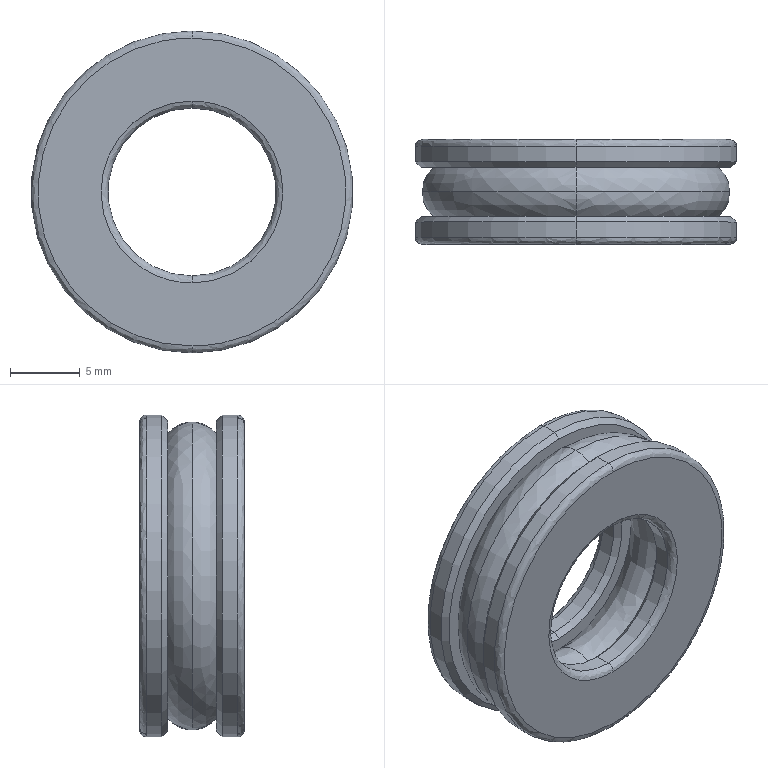Part | SolidWorks | features BaseBody 1 | 1 solid | 36 faces | box 23 x 7.5 x 23 mm | volume 1948 mm3 | spline 14 | cylinder 8 | cone 8 | plane 6 | commonest cylinder face diameters 12 x4 23 x4
STEP:
#1=CARTESIAN_POINT('',(0.,0.5,-6.));
#2=VERTEX_POINT('',#1);
#3=CARTESIAN_POINT('',(0.,0.5,6.));
#4=VERTEX_POINT('',#3);
#5=CARTESIAN_POINT('',(0.,0.5,0.));
#6=DIRECTION('',(0.,1.,0.));
#7=DIRECTION('',(0.,0.,-1.));
#8=AXIS2_PLACEMENT_3D('',#5,#6,#7);
#9=CIRCLE('',#8,6.);
#10=EDGE_CURVE('',#2,#4,#9,.T.);
#11=ORIENTED_EDGE('',*,*,#10,.T.);
#12=CARTESIAN_POINT('',(0.,0.,6.5));
#13=VERTEX_POINT('',#12);
#14=CARTESIAN_POINT('',(0.,0.5,6.5));
#15=DIRECTION('',(-1.,0.,0.));
#16=DIRECTION('',(0.,0.,1.));
#17=AXIS2_PLACEMENT_3D('',#14,#15,#16);
#18=CIRCLE('',#17,0.5);
#19=EDGE_CURVE('',#4,#13,#18,.T.);
#20=ORIENTED_EDGE('',*,*,#19,.T.);
#21=CARTESIAN_POINT('',(0.,0.,-6.5));
#22=VERTEX_POINT('',#21);
#23=CARTESIAN_POINT('',(0.,0.,6.5));
#24=CARTESIAN_POINT('',(-13.,0.,6.5));
#25=CARTESIAN_POINT('',(-13.,0.,-6.5));
#26=CARTESIAN_POINT('',(0.,0.,-6.5));
#27=(BOUNDED_CURVE()B_SPLINE_CURVE(3,(#23,#24,#25,#26),.UNSPECIFIED.,.F.,.F.)B_SPLINE_CURVE_WITH_KNOTS((4,4),(0.,1.),.UNSPECIFIED.)CURVE()GEOMETRIC_REPRESENTATION_ITEM()RATIONAL_B_SPLINE_CURVE((1.,0.3333,0.3333,1.))REPRESENTATION_ITEM(''));
#28=EDGE_CURVE('',#13,#22,#27,.T.);
#29=ORIENTED_EDGE('',*,*,#28,.T.);
#30=CARTESIAN_POINT('',(0.,0.5,-6.5));
#31=DIRECTION('',(1.,0.,0.));
#32=DIRECTION('',(0.,0.,-1.));
#33=AXIS2_PLACEMENT_3D('',#30,#31,#32);
#34=CIRCLE('',#33,0.5);
#35=EDGE_CURVE('',#2,#22,#34,.T.);
#36=ORIENTED_EDGE('',*,*,#35,.F.);
#37=EDGE_LOOP('',(#11,#20,#29,#36));
#38=FACE_OUTER_BOUND('',#37,.T.);
#39=CARTESIAN_POINT('',(0.,0.5,6.));
#40=CARTESIAN_POINT('',(-12.,0.5,6.));
#41=CARTESIAN_POINT('',(-12.,0.5,-6.));
#42=CARTESIAN_POINT('',(0.,0.5,-6.));
#43=CARTESIAN_POINT('',(0.,0.2071,6.));
#44=CARTESIAN_POINT('',(-12.,0.2071,6.));
#45=CARTESIAN_POINT('',(-12.,0.2071,-6.));
#46=CARTESIAN_POINT('',(0.,0.2071,-6.));
#47=CARTESIAN_POINT('',(0.,0.,6.207));
#48=CARTESIAN_POINT('',(-12.414,0.,6.207));
#49=CARTESIAN_POINT('',(-12.414,0.,-6.207));
#50=CARTESIAN_POINT('',(0.,0.,-6.207));
#51=CARTESIAN_POINT('',(0.,0.,6.5));
#52=CARTESIAN_POINT('',(-13.,0.,6.5));
#53=CARTESIAN_POINT('',(-13.,0.,-6.5));
#54=CARTESIAN_POINT('',(0.,0.,-6.5));
#55=(BOUNDED_SURFACE()B_SPLINE_SURFACE(3,3,((#39,#40,#41,#42),(#43,#44,#45,#46),(#47,#48,#49,#50),(#51,#52,#53,#54)),.UNSPECIFIED.,.F.,.F.,.F.)B_SPLINE_SURFACE_WITH_KNOTS((4,4),(4,4),(0.,1.),(0.,1.),.UNSPECIFIED.)GEOMETRIC_REPRESENTATION_ITEM()RATIONAL_B_SPLINE_SURFACE(((1.,0.3333,0.3333,1.),(0.8047,0.2682,0.2682,0.8047),(0.8047,0.2682,0.2682,0.8047),(1.,0.3333,0.3333,1.)))REPRESENTATION_ITEM('')SURFACE());
#56=ADVANCED_FACE('',(#38),#55,.T.);
#57=CARTESIAN_POINT('',(0.,0.,-11.));
#58=VERTEX_POINT('',#57);
#59=CARTESIAN_POINT('',(0.,0.,11.));
#60=VERTEX_POINT('',#59);
#61=CARTESIAN_POINT('',(0.,0.,-11.));
#62=CARTESIAN_POINT('',(-22.,0.,-11.));
#63=CARTESIAN_POINT('',(-22.,0.,11.));
#64=CARTESIAN_POINT('',(0.,0.,11.));
#65=(BOUNDED_CURVE()B_SPLINE_CURVE(3,(#61,#62,#63,#64),.UNSPECIFIED.,.F.,.F.)B_SPLINE_CURVE_WITH_KNOTS((4,4),(0.,1.),.UNSPECIFIED.)CURVE()GEOMETRIC_REPRESENTATION_ITEM()RATIONAL_B_SPLINE_CURVE((1.,0.3333,0.3333,1.))REPRESENTATION_ITEM(''));
#66=EDGE_CURVE('',#58,#60,#65,.T.);
#67=ORIENTED_EDGE('',*,*,#66,.T.);
#68=CARTESIAN_POINT('',(0.,0.5,11.5));
#69=VERTEX_POINT('',#68);
#70=CARTESIAN_POINT('',(0.,0.5,11.));
#71=DIRECTION('',(-1.,0.,0.));
#72=DIRECTION('',(0.,0.,1.));
#73=AXIS2_PLACEMENT_3D('',#70,#71,#72);
#74=CIRCLE('',#73,0.5);
#75=EDGE_CURVE('',#60,#69,#74,.T.);
#76=ORIENTED_EDGE('',*,*,#75,.T.);
#77=CARTESIAN_POINT('',(0.,0.5,-11.5));
#78=VERTEX_POINT('',#77);
#79=CARTESIAN_POINT('',(0.,0.5,0.));
#80=DIRECTION('',(0.,-1.,0.));
#81=DIRECTION('',(0.,0.,-1.));
#82=AXIS2_PLACEMENT_3D('',#79,#80,#81);
#83=CIRCLE('',#82,11.5);
#84=EDGE_CURVE('',#69,#78,#83,.T.);
#85=ORIENTED_EDGE('',*,*,#84,.T.);
#86=CARTESIAN_POINT('',(0.,0.5,-11.));
#87=DIRECTION('',(1.,0.,0.));
#88=DIRECTION('',(0.,0.,-1.));
#89=AXIS2_PLACEMENT_3D('',#86,#87,#88);
#90=CIRCLE('',#89,0.5);
#91=EDGE_CURVE('',#58,#78,#90,.T.);
#92=ORIENTED_EDGE('',*,*,#91,.F.);
#93=EDGE_LOOP('',(#67,#76,#85,#92));
#94=FACE_OUTER_BOUND('',#93,.T.);
#95=CARTESIAN_POINT('',(0.,0.,11.));
#96=CARTESIAN_POINT('',(-22.,0.,11.));
#97=CARTESIAN_POINT('',(-22.,0.,-11.));
#98=CARTESIAN_POINT('',(0.,0.,-11.));
#99=CARTESIAN_POINT('',(0.,0.,11.293));
#100=CARTESIAN_POINT('',(-22.586,0.,11.293));
#101=CARTESIAN_POINT('',(-22.586,0.,-11.293));
#102=CARTESIAN_POINT('',(0.,0.,-11.293));
#103=CARTESIAN_POINT('',(0.,0.2071,11.5));
#104=CARTESIAN_POINT('',(-23.,0.2071,11.5));
#105=CARTESIAN_POINT('',(-23.,0.2071,-11.5));
#106=CARTESIAN_POINT('',(0.,0.2071,-11.5));
#107=CARTESIAN_POINT('',(0.,0.5,11.5));
#108=CARTESIAN_POINT('',(-23.,0.5,11.5));
#109=CARTESIAN_POINT('',(-23.,0.5,-11.5));
#110=CARTESIAN_POINT('',(0.,0.5,-11.5));
#111=(BOUNDED_SURFACE()B_SPLINE_SURFACE(3,3,((#95,#96,#97,#98),(#99,#100,#101,#102),(#103,#104,#105,#106),(#107,#108,#109,#110)),.UNSPECIFIED.,.F.,.F.,.F.)B_SPLINE_SURFACE_WITH_KNOTS((4,4),(4,4),(0.,1.),(0.,1.),.UNSPECIFIED.)GEOMETRIC_REPRESENTATION_ITEM()RATIONAL_B_SPLINE_SURFACE(((1.,0.3333,0.3333,1.),(0.8047,0.2682,0.2682,0.8047),(0.8047,0.2682,0.2682,0.8047),(1.,0.3333,0.3333,1.)))REPRESENTATION_ITEM('')SURFACE());
#112=ADVANCED_FACE('',(#94),#111,.T.);
#113=CARTESIAN_POINT('',(0.,5.5,7.336));
#114=VERTEX_POINT('',#113);
#115=CARTESIAN_POINT('',(0.,5.5,-7.336));
#116=VERTEX_POINT('',#115);
#117=CARTESIAN_POINT('',(0.,5.5,0.));
#118=DIRECTION('',(0.,1.,0.));
#119=DIRECTION('',(0.,0.,-1.));
#120=AXIS2_PLACEMENT_3D('',#117,#118,#119);
#121=CIRCLE('',#120,7.336);
#122=EDGE_CURVE('',#114,#116,#121,.T.);
#123=ORIENTED_EDGE('',*,*,#122,.T.);
#124=CARTESIAN_POINT('',(0.,2.,-7.336));
#125=VERTEX_POINT('',#124);
#126=CARTESIAN_POINT('',(0.,3.75,-8.75));
#127=DIRECTION('',(1.,0.,0.));
#128=DIRECTION('',(0.,0.,-1.));
#129=AXIS2_PLACEMENT_3D('',#126,#127,#128);
#130=CIRCLE('',#129,2.25);
#131=EDGE_CURVE('',#116,#125,#130,.T.);
#132=ORIENTED_EDGE('',*,*,#131,.T.);
#133=CARTESIAN_POINT('',(0.,2.,7.336));
#134=VERTEX_POINT('',#133);
#135=CARTESIAN_POINT('',(0.,2.,0.));
#136=DIRECTION('',(0.,1.,0.));
#137=DIRECTION('',(0.,0.,-1.));
#138=AXIS2_PLACEMENT_3D('',#135,#136,#137);
#139=CIRCLE('',#138,7.336);
#140=EDGE_CURVE('',#134,#125,#139,.T.);
#141=ORIENTED_EDGE('',*,*,#140,.F.);
#142=CARTESIAN_POINT('',(0.,3.75,8.75));
#143=DIRECTION('',(-1.,0.,0.));
#144=DIRECTION('',(0.,0.,1.));
#145=AXIS2_PLACEMENT_3D('',#142,#143,#144);
#146=CIRCLE('',#145,2.25);
#147=EDGE_CURVE('',#114,#134,#146,.T.);
#148=ORIENTED_EDGE('',*,*,#147,.F.);
#149=EDGE_LOOP('',(#123,#132,#141,#148));
#150=FACE_OUTER_BOUND('',#149,.T.);
#151=CARTESIAN_POINT('',(0.,5.5,-7.336));
#152=CARTESIAN_POINT('',(14.672,5.5,-7.336));
#153=CARTESIAN_POINT('',(14.672,5.5,7.336));
#154=CARTESIAN_POINT('',(0.,5.5,7.336));
#155=CARTESIAN_POINT('',(0.,4.525,-6.13));
#156=CARTESIAN_POINT('',(12.259,4.525,-6.13));
#157=CARTESIAN_POINT('',(12.259,4.525,6.13));
#158=CARTESIAN_POINT('',(0.,4.525,6.13));
#159=CARTESIAN_POINT('',(0.,2.975,-6.13));
#160=CARTESIAN_POINT('',(12.259,2.975,-6.13));
#161=CARTESIAN_POINT('',(12.259,2.975,6.13));
#162=CARTESIAN_POINT('',(0.,2.975,6.13));
#163=CARTESIAN_POINT('',(0.,2.,-7.336));
#164=CARTESIAN_POINT('',(14.672,2.,-7.336));
#165=CARTESIAN_POINT('',(14.672,2.,7.336));
#166=CARTESIAN_POINT('',(0.,2.,7.336));
#167=(BOUNDED_SURFACE()B_SPLINE_SURFACE(3,3,((#151,#152,#153,#154),(#155,#156,#157,#158),(#159,#160,#161,#162),(#163,#164,#165,#166)),.UNSPECIFIED.,.F.,.F.,.F.)B_SPLINE_SURFACE_WITH_KNOTS((4,4),(4,4),(0.,1.),(0.,1.),.UNSPECIFIED.)GEOMETRIC_REPRESENTATION_ITEM()RATIONAL_B_SPLINE_SURFACE(((1.,0.3333,0.3333,1.),(0.7524,0.2508,0.2508,0.7524),(0.7524,0.2508,0.2508,0.7524),(1.,0.3333,0.3333,1.)))REPRESENTATION_ITEM('')SURFACE());
#168=ADVANCED_FACE('',(#150),#167,.T.);
#169=CARTESIAN_POINT('',(0.,3.75,11.));
#170=VERTEX_POINT('',#169);
#171=CARTESIAN_POINT('',(0.,3.75,-11.));
#172=VERTEX_POINT('',#171);
#173=CARTESIAN_POINT('',(0.,3.75,0.));
#174=DIRECTION('',(0.,-1.,0.));
#175=DIRECTION('',(0.,0.,-1.));
#176=AXIS2_PLACEMENT_3D('',#173,#174,#175);
#177=CIRCLE('',#176,11.);
#178=EDGE_CURVE('',#170,#172,#177,.T.);
#179=ORIENTED_EDGE('',*,*,#178,.F.);
#180=CARTESIAN_POINT('',(0.,5.5,10.164));
#181=VERTEX_POINT('',#180);
#182=CARTESIAN_POINT('',(0.,3.75,8.75));
#183=DIRECTION('',(-1.,0.,0.));
#184=DIRECTION('',(0.,0.,1.));
#185=AXIS2_PLACEMENT_3D('',#182,#183,#184);
#186=CIRCLE('',#185,2.25);
#187=EDGE_CURVE('',#170,#181,#186,.T.);
#188=ORIENTED_EDGE('',*,*,#187,.T.);
#189=CARTESIAN_POINT('',(0.,5.5,-10.164));
#190=VERTEX_POINT('',#189);
#191=CARTESIAN_POINT('',(0.,5.5,0.));
#192=DIRECTION('',(0.,-1.,0.));
#193=DIRECTION('',(0.,0.,-1.));
#194=AXIS2_PLACEMENT_3D('',#191,#192,#193);
#195=CIRCLE('',#194,10.164);
#196=EDGE_CURVE('',#181,#190,#195,.T.);
#197=ORIENTED_EDGE('',*,*,#196,.T.);
#198=CARTESIAN_POINT('',(0.,3.75,-8.75));
#199=DIRECTION('',(1.,0.,0.));
#200=DIRECTION('',(0.,0.,-1.));
#201=AXIS2_PLACEMENT_3D('',#198,#199,#200);
#202=CIRCLE('',#201,2.25);
#203=EDGE_CURVE('',#172,#190,#202,.T.);
#204=ORIENTED_EDGE('',*,*,#203,.F.);
#205=EDGE_LOOP('',(#179,#188,#197,#204));
#206=FACE_OUTER_BOUND('',#205,.T.);
#207=CARTESIAN_POINT('',(0.,3.75,11.));
#208=CARTESIAN_POINT('',(-22.,3.75,11.));
#209=CARTESIAN_POINT('',(-22.,3.75,-11.));
#210=CARTESIAN_POINT('',(0.,3.75,-11.));
#211=CARTESIAN_POINT('',(0.,4.441,11.));
#212=CARTESIAN_POINT('',(-22.,4.441,11.));
#213=CARTESIAN_POINT('',(-22.,4.441,-11.));
#214=CARTESIAN_POINT('',(0.,4.441,-11.));
#215=CARTESIAN_POINT('',(0.,5.065,10.702));
#216=CARTESIAN_POINT('',(-21.404,5.065,10.702));
#217=CARTESIAN_POINT('',(-21.404,5.065,-10.702));
#218=CARTESIAN_POINT('',(0.,5.065,-10.702));
#219=CARTESIAN_POINT('',(0.,5.5,10.164));
#220=CARTESIAN_POINT('',(-20.328,5.5,10.164));
#221=CARTESIAN_POINT('',(-20.328,5.5,-10.164));
#222=CARTESIAN_POINT('',(0.,5.5,-10.164));
#223=(BOUNDED_SURFACE()B_SPLINE_SURFACE(3,3,((#207,#208,#209,#210),(#211,#212,#213,#214),(#215,#216,#217,#218),(#219,#220,#221,#222)),.UNSPECIFIED.,.F.,.F.,.F.)B_SPLINE_SURFACE_WITH_KNOTS((4,4),(4,4),(0.,1.),(0.,1.),.UNSPECIFIED.)GEOMETRIC_REPRESENTATION_ITEM()RATIONAL_B_SPLINE_SURFACE(((1.,0.3333,0.3333,1.),(0.9349,0.3116,0.3116,0.9349),(0.9349,0.3116,0.3116,0.9349),(1.,0.3333,0.3333,1.)))REPRESENTATION_ITEM('')SURFACE());
#224=ADVANCED_FACE('',(#206),#223,.T.);
#225=CARTESIAN_POINT('',(0.,7.5,6.5));
#226=VERTEX_POINT('',#225);
#227=CARTESIAN_POINT('',(0.,7.5,-6.5));
#228=VERTEX_POINT('',#227);
#229=CARTESIAN_POINT('',(0.,7.5,6.5));
#230=CARTESIAN_POINT('',(13.,7.5,6.5));
#231=CARTESIAN_POINT('',(13.,7.5,-6.5));
#232=CARTESIAN_POINT('',(0.,7.5,-6.5));
#233=(BOUNDED_CURVE()B_SPLINE_CURVE(3,(#229,#230,#231,#232),.UNSPECIFIED.,.F.,.F.)B_SPLINE_CURVE_WITH_KNOTS((4,4),(0.,1.),.UNSPECIFIED.)CURVE()GEOMETRIC_REPRESENTATION_ITEM()RATIONAL_B_SPLINE_CURVE((1.,0.3333,0.3333,1.))REPRESENTATION_ITEM(''));
#234=EDGE_CURVE('',#226,#228,#233,.T.);
#235=ORIENTED_EDGE('',*,*,#234,.T.);
#236=CARTESIAN_POINT('',(0.,7.,-6.));
#237=VERTEX_POINT('',#236);
#238=CARTESIAN_POINT('',(0.,7.,-6.5));
#239=DIRECTION('',(1.,0.,0.));
#240=DIRECTION('',(0.,0.,-1.));
#241=AXIS2_PLACEMENT_3D('',#238,#239,#240);
#242=CIRCLE('',#241,0.5);
#243=EDGE_CURVE('',#228,#237,#242,.T.);
#244=ORIENTED_EDGE('',*,*,#243,.T.);
#245=CARTESIAN_POINT('',(0.,7.,6.));
#246=VERTEX_POINT('',#245);
#247=CARTESIAN_POINT('',(0.,7.,0.));
#248=DIRECTION('',(0.,-1.,0.));
#249=DIRECTION('',(0.,0.,-1.));
#250=AXIS2_PLACEMENT_3D('',#247,#248,#249);
#251=CIRCLE('',#250,6.);
#252=EDGE_CURVE('',#237,#246,#251,.T.);
#253=ORIENTED_EDGE('',*,*,#252,.T.);
#254=CARTESIAN_POINT('',(0.,7.,6.5));
#255=DIRECTION('',(-1.,0.,0.));
#256=DIRECTION('',(0.,0.,1.));
#257=AXIS2_PLACEMENT_3D('',#254,#255,#256);
#258=CIRCLE('',#257,0.5);
#259=EDGE_CURVE('',#226,#246,#258,.T.);
#260=ORIENTED_EDGE('',*,*,#259,.F.);
#261=EDGE_LOOP('',(#235,#244,#253,#260));
#262=FACE_OUTER_BOUND('',#261,.T.);
#263=CARTESIAN_POINT('',(0.,7.5,-6.5));
#264=CARTESIAN_POINT('',(13.,7.5,-6.5));
#265=CARTESIAN_POINT('',(13.,7.5,6.5));
#266=CARTESIAN_POINT('',(0.,7.5,6.5));
#267=CARTESIAN_POINT('',(0.,7.5,-6.207));
#268=CARTESIAN_POINT('',(12.414,7.5,-6.207));
#269=CARTESIAN_POINT('',(12.414,7.5,6.207));
#270=CARTESIAN_POINT('',(0.,7.5,6.207));
#271=CARTESIAN_POINT('',(0.,7.293,-6.));
#272=CARTESIAN_POINT('',(12.,7.293,-6.));
#273=CARTESIAN_POINT('',(12.,7.293,6.));
#274=CARTESIAN_POINT('',(0.,7.293,6.));
#275=CARTESIAN_POINT('',(0.,7.,-6.));
#276=CARTESIAN_POINT('',(12.,7.,-6.));
#277=CARTESIAN_POINT('',(12.,7.,6.));
#278=CARTESIAN_POINT('',(0.,7.,6.));
#279=(BOUNDED_SURFACE()B_SPLINE_SURFACE(3,3,((#263,#264,#265,#266),(#267,#268,#269,#270),(#271,#272,#273,#274),(#275,#276,#277,#278)),.UNSPECIFIED.,.F.,.F.,.F.)B_SPLINE_SURFACE_WITH_KNOTS((4,4),(4,4),(0.,1.),(0.,1.),.UNSPECIFIED.)GEOMETRIC_REPRESENTATION_ITEM()RATIONAL_B_SPLINE_SURFACE(((1.,0.3333,0.3333,1.),(0.8047,0.2682,0.2682,0.8047),(0.8047,0.2682,0.2682,0.8047),(1.,0.3333,0.3333,1.)))REPRESENTATION_ITEM('')SURFACE());
#280=ADVANCED_FACE('',(#262),#279,.T.);
#281=CARTESIAN_POINT('',(0.,7.,-11.5));
#282=VERTEX_POINT('',#281);
#283=CARTESIAN_POINT('',(0.,7.,11.5));
#284=VERTEX_POINT('',#283);
#285=CARTESIAN_POINT('',(0.,7.,0.));
#286=DIRECTION('',(0.,-1.,0.));
#287=DIRECTION('',(0.,0.,-1.));
#288=AXIS2_PLACEMENT_3D('',#285,#286,#287);
#289=CIRCLE('',#288,11.5);
#290=EDGE_CURVE('',#282,#284,#289,.T.);
#291=ORIENTED_EDGE('',*,*,#290,.F.);
#292=CARTESIAN_POINT('',(0.,7.5,-11.));
#293=VERTEX_POINT('',#292);
#294=CARTESIAN_POINT('',(0.,7.,-11.));
#295=DIRECTION('',(1.,0.,0.));
#296=DIRECTION('',(0.,0.,-1.));
#297=AXIS2_PLACEMENT_3D('',#294,#295,#296);
#298=CIRCLE('',#297,0.5);
#299=EDGE_CURVE('',#282,#293,#298,.T.);
#300=ORIENTED_EDGE('',*,*,#299,.T.);
#301=CARTESIAN_POINT('',(0.,7.5,11.));
#302=VERTEX_POINT('',#301);
#303=CARTESIAN_POINT('',(0.,7.5,-11.));
#304=CARTESIAN_POINT('',(22.,7.5,-11.));
#305=CARTESIAN_POINT('',(22.,7.5,11.));
#306=CARTESIAN_POINT('',(0.,7.5,11.));
#307=(BOUNDED_CURVE()B_SPLINE_CURVE(3,(#303,#304,#305,#306),.UNSPECIFIED.,.F.,.F.)B_SPLINE_CURVE_WITH_KNOTS((4,4),(0.,1.),.UNSPECIFIED.)CURVE()GEOMETRIC_REPRESENTATION_ITEM()RATIONAL_B_SPLINE_CURVE((1.,0.3333,0.3333,1.))REPRESENTATION_ITEM(''));
#308=EDGE_CURVE('',#293,#302,#307,.T.);
#309=ORIENTED_EDGE('',*,*,#308,.T.);
#310=CARTESIAN_POINT('',(0.,7.,11.));
#311=DIRECTION('',(-1.,0.,0.));
#312=DIRECTION('',(0.,0.,1.));
#313=AXIS2_PLACEMENT_3D('',#310,#311,#312);
#314=CIRCLE('',#313,0.5);
#315=EDGE_CURVE('',#284,#302,#314,.T.);
#316=ORIENTED_EDGE('',*,*,#315,.F.);
#317=EDGE_LOOP('',(#291,#300,#309,#316));
#318=FACE_OUTER_BOUND('',#317,.T.);
#319=CARTESIAN_POINT('',(0.,7.,-11.5));
#320=CARTESIAN_POINT('',(23.,7.,-11.5));
#321=CARTESIAN_POINT('',(23.,7.,11.5));
#322=CARTESIAN_POINT('',(0.,7.,11.5));
#323=CARTESIAN_POINT('',(0.,7.293,-11.5));
#324=CARTESIAN_POINT('',(23.,7.293,-11.5));
#325=CARTESIAN_POINT('',(23.,7.293,11.5));
#326=CARTESIAN_POINT('',(0.,7.293,11.5));
#327=CARTESIAN_POINT('',(0.,7.5,-11.293));
#328=CARTESIAN_POINT('',(22.586,7.5,-11.293));
#329=CARTESIAN_POINT('',(22.586,7.5,11.293));
#330=CARTESIAN_POINT('',(0.,7.5,11.293));
#331=CARTESIAN_POINT('',(0.,7.5,-11.));
#332=CARTESIAN_POINT('',(22.,7.5,-11.));
#333=CARTESIAN_POINT('',(22.,7.5,11.));
#334=CARTESIAN_POINT('',(0.,7.5,11.));
#335=(BOUNDED_SURFACE()B_SPLINE_SURFACE(3,3,((#319,#320,#321,#322),(#323,#324,#325,#326),(#327,#328,#329,#330),(#331,#332,#333,#334)),.UNSPECIFIED.,.F.,.F.,.F.)B_SPLINE_SURFACE_WITH_KNOTS((4,4),(4,4),(0.,1.),(0.,1.),.UNSPECIFIED.)GEOMETRIC_REPRESENTATION_ITEM()RATIONAL_B_SPLINE_SURFACE(((1.,0.3333,0.3333,1.),(0.8047,0.2682,0.2682,0.8047),(0.8047,0.2682,0.2682,0.8047),(1.,0.3333,0.3333,1.)))REPRESENTATION_ITEM('')SURFACE());
#336=ADVANCED_FACE('',(#318),#335,.T.);
#337=CARTESIAN_POINT('',(0.,2.,-10.164));
#338=VERTEX_POINT('',#337);
#339=CARTESIAN_POINT('',(0.,2.,10.164));
#340=VERTEX_POINT('',#339);
#341=CARTESIAN_POINT('',(0.,2.,0.));
#342=DIRECTION('',(0.,1.,0.));
#343=DIRECTION('',(0.,0.,-1.));
#344=AXIS2_PLACEMENT_3D('',#341,#342,#343);
#345=CIRCLE('',#344,10.164);
#346=EDGE_CURVE('',#338,#340,#345,.T.);
#347=ORIENTED_EDGE('',*,*,#346,.T.);
#348=CARTESIAN_POINT('',(0.,3.75,8.75));
#349=DIRECTION('',(-1.,0.,0.));
#350=DIRECTION('',(0.,0.,1.));
#351=AXIS2_PLACEMENT_3D('',#348,#349,#350);
#352=CIRCLE('',#351,2.25);
#353=EDGE_CURVE('',#340,#170,#352,.T.);
#354=ORIENTED_EDGE('',*,*,#353,.T.);
#355=ORIENTED_EDGE('',*,*,#178,.T.);
#356=CARTESIAN_POINT('',(0.,3.75,-8.75));
#357=DIRECTION('',(1.,0.,0.));
#358=DIRECTION('',(0.,0.,-1.));
#359=AXIS2_PLACEMENT_3D('',#356,#357,#358);
#360=CIRCLE('',#359,2.25);
#361=EDGE_CURVE('',#338,#172,#360,.T.);
#362=ORIENTED_EDGE('',*,*,#361,.F.);
#363=EDGE_LOOP('',(#347,#354,#355,#362));
#364=FACE_OUTER_BOUND('',#363,.T.);
#365=CARTESIAN_POINT('',(0.,2.,10.164));
#366=CARTESIAN_POINT('',(-20.328,2.,10.164));
#367=CARTESIAN_POINT('',(-20.328,2.,-10.164));
#368=CARTESIAN_POINT('',(0.,2.,-10.164));
#369=CARTESIAN_POINT('',(0.,2.435,10.702));
#370=CARTESIAN_POINT('',(-21.404,2.435,10.702));
#371=CARTESIAN_POINT('',(-21.404,2.435,-10.702));
#372=CARTESIAN_POINT('',(0.,2.435,-10.702));
#373=CARTESIAN_POINT('',(0.,3.059,11.));
#374=CARTESIAN_POINT('',(-22.,3.059,11.));
#375=CARTESIAN_POINT('',(-22.,3.059,-11.));
#376=CARTESIAN_POINT('',(0.,3.059,-11.));
#377=CARTESIAN_POINT('',(0.,3.75,11.));
#378=CARTESIAN_POINT('',(-22.,3.75,11.));
#379=CARTESIAN_POINT('',(-22.,3.75,-11.));
#380=CARTESIAN_POINT('',(0.,3.75,-11.));
#381=(BOUNDED_SURFACE()B_SPLINE_SURFACE(3,3,((#365,#366,#367,#368),(#369,#370,#371,#372),(#373,#374,#375,#376),(#377,#378,#379,#380)),.UNSPECIFIED.,.F.,.F.,.F.)B_SPLINE_SURFACE_WITH_KNOTS((4,4),(4,4),(0.,1.),(0.,1.),.UNSPECIFIED.)GEOMETRIC_REPRESENTATION_ITEM()RATIONAL_B_SPLINE_SURFACE(((1.,0.3333,0.3333,1.),(0.9349,0.3116,0.3116,0.9349),(0.9349,0.3116,0.3116,0.9349),(1.,0.3333,0.3333,1.)))REPRESENTATION_ITEM('')SURFACE());
#382=ADVANCED_FACE('',(#364),#381,.T.);
#383=CARTESIAN_POINT('',(0.,1.6,6.));
#384=VERTEX_POINT('',#383);
#385=CARTESIAN_POINT('',(0.,1.6,-6.));
#386=VERTEX_POINT('',#385);
#387=CARTESIAN_POINT('',(0.,1.6,0.));
#388=DIRECTION('',(0.,-1.,0.));
#389=DIRECTION('',(0.,0.,-1.));
#390=AXIS2_PLACEMENT_3D('',#387,#388,#389);
#391=CIRCLE('',#390,6.);
#392=EDGE_CURVE('',#384,#386,#391,.T.);
#393=ORIENTED_EDGE('',*,*,#392,.F.);
#394=CARTESIAN_POINT('',(0.,0.,6.));
#395=DIRECTION('',(0.,-1.,0.));
#396=VECTOR('',#395,1000.);
#397=LINE('',#394,#396);
#398=EDGE_CURVE('',#384,#4,#397,.T.);
#399=ORIENTED_EDGE('',*,*,#398,.T.);
#400=ORIENTED_EDGE('',*,*,#10,.F.);
#401=CARTESIAN_POINT('',(0.,0.,-6.));
#402=DIRECTION('',(0.,-1.,0.));
#403=VECTOR('',#402,1000.);
#404=LINE('',#401,#403);
#405=EDGE_CURVE('',#386,#2,#404,.T.);
#406=ORIENTED_EDGE('',*,*,#405,.F.);
#407=EDGE_LOOP('',(#393,#399,#400,#406));
#408=FACE_OUTER_BOUND('',#407,.T.);
#409=CARTESIAN_POINT('',(0.,0.,0.));
#410=DIRECTION('',(0.,-1.,0.));
#411=DIRECTION('',(0.,0.,-1.));
#412=AXIS2_PLACEMENT_3D('',#409,#410,#411);
#413=CYLINDRICAL_SURFACE('',#412,6.);
#414=ADVANCED_FACE('',(#408),#413,.F.);
#415=CARTESIAN_POINT('',(0.,1.6,-11.5));
#416=VERTEX_POINT('',#415);
#417=CARTESIAN_POINT('',(0.,1.6,11.5));
#418=VERTEX_POINT('',#417);
#419=CARTESIAN_POINT('',(0.,1.6,0.));
#420=DIRECTION('',(0.,-1.,0.));
#421=DIRECTION('',(0.,0.,-1.));
#422=AXIS2_PLACEMENT_3D('',#419,#420,#421);
#423=CIRCLE('',#422,11.5);
#424=EDGE_CURVE('',#416,#418,#423,.T.);
#425=ORIENTED_EDGE('',*,*,#424,.T.);
#426=CARTESIAN_POINT('',(0.,0.,11.5));
#427=DIRECTION('',(0.,-1.,0.));
#428=VECTOR('',#427,1000.);
#429=LINE('',#426,#428);
#430=EDGE_CURVE('',#418,#69,#429,.T.);
#431=ORIENTED_EDGE('',*,*,#430,.T.);
#432=CARTESIAN_POINT('',(0.,0.5,0.));
#433=DIRECTION('',(0.,-1.,0.));
#434=DIRECTION('',(0.,0.,-1.));
#435=AXIS2_PLACEMENT_3D('',#432,#433,#434);
#436=CIRCLE('',#435,11.5);
#437=EDGE_CURVE('',#78,#69,#436,.T.);
#438=ORIENTED_EDGE('',*,*,#437,.F.);
#439=CARTESIAN_POINT('',(0.,0.,-11.5));
#440=DIRECTION('',(0.,-1.,0.));
#441=VECTOR('',#440,1000.);
#442=LINE('',#439,#441);
#443=EDGE_CURVE('',#416,#78,#442,.T.);
#444=ORIENTED_EDGE('',*,*,#443,.F.);
#445=EDGE_LOOP('',(#425,#431,#438,#444));
#446=FACE_OUTER_BOUND('',#445,.T.);
#447=CARTESIAN_POINT('',(0.,0.,0.));
#448=DIRECTION('',(0.,-1.,0.));
#449=DIRECTION('',(0.,0.,-1.));
#450=AXIS2_PLACEMENT_3D('',#447,#448,#449);
#451=CYLINDRICAL_SURFACE('',#450,11.5);
#452=ADVANCED_FACE('',(#446),#451,.T.);
#453=ORIENTED_EDGE('',*,*,#392,.T.);
#454=CARTESIAN_POINT('',(0.,2.,-6.4));
#455=VERTEX_POINT('',#454);
#456=CARTESIAN_POINT('',(0.,2.,-6.4));
#457=DIRECTION('',(0.,0.7071,-0.7071));
#458=VECTOR('',#457,1000.);
#459=LINE('',#456,#458);
#460=EDGE_CURVE('',#386,#455,#459,.T.);
#461=ORIENTED_EDGE('',*,*,#460,.T.);
#462=CARTESIAN_POINT('',(0.,2.,6.4));
#463=VERTEX_POINT('',#462);
#464=CARTESIAN_POINT('',(0.,2.,0.));
#465=DIRECTION('',(0.,-1.,0.));
#466=DIRECTION('',(0.,0.,1.));
#467=AXIS2_PLACEMENT_3D('',#464,#465,#466);
#468=CIRCLE('',#467,6.4);
#469=EDGE_CURVE('',#463,#455,#468,.T.);
#470=ORIENTED_EDGE('',*,*,#469,.F.);
#471=CARTESIAN_POINT('',(0.,2.,6.4));
#472=DIRECTION('',(0.,0.7071,0.7071));
#473=VECTOR('',#472,1000.);
#474=LINE('',#471,#473);
#475=EDGE_CURVE('',#384,#463,#474,.T.);
#476=ORIENTED_EDGE('',*,*,#475,.F.);
#477=EDGE_LOOP('',(#453,#461,#470,#476));
#478=FACE_OUTER_BOUND('',#477,.T.);
#479=CARTESIAN_POINT('',(0.,2.,0.));
#480=DIRECTION('',(0.,1.,0.));
#481=DIRECTION('',(0.,0.,1.));
#482=AXIS2_PLACEMENT_3D('',#479,#480,#481);
#483=CONICAL_SURFACE('',#482,6.4,0.7854);
#484=ADVANCED_FACE('',(#478),#483,.F.);
#485=CARTESIAN_POINT('',(0.,2.,-11.1));
#486=VERTEX_POINT('',#485);
#487=CARTESIAN_POINT('',(0.,2.,11.1));
#488=VERTEX_POINT('',#487);
#489=CARTESIAN_POINT('',(0.,2.,0.));
#490=DIRECTION('',(0.,-1.,0.));
#491=DIRECTION('',(0.,0.,-1.));
#492=AXIS2_PLACEMENT_3D('',#489,#490,#491);
#493=CIRCLE('',#492,11.1);
#494=EDGE_CURVE('',#486,#488,#493,.T.);
#495=ORIENTED_EDGE('',*,*,#494,.T.);
#496=CARTESIAN_POINT('',(0.,1.6,11.5));
#497=DIRECTION('',(0.,-0.7071,0.7071));
#498=VECTOR('',#497,1000.);
#499=LINE('',#496,#498);
#500=EDGE_CURVE('',#488,#418,#499,.T.);
#501=ORIENTED_EDGE('',*,*,#500,.T.);
#502=ORIENTED_EDGE('',*,*,#424,.F.);
#503=CARTESIAN_POINT('',(0.,1.6,-11.5));
#504=DIRECTION('',(0.,-0.7071,-0.7071));
#505=VECTOR('',#504,1000.);
#506=LINE('',#503,#505);
#507=EDGE_CURVE('',#486,#416,#506,.T.);
#508=ORIENTED_EDGE('',*,*,#507,.F.);
#509=EDGE_LOOP('',(#495,#501,#502,#508));
#510=FACE_OUTER_BOUND('',#509,.T.);
#511=CARTESIAN_POINT('',(0.,1.6,0.));
#512=DIRECTION('',(0.,-1.,0.));
#513=DIRECTION('',(0.,0.,-1.));
#514=AXIS2_PLACEMENT_3D('',#511,#512,#513);
#515=CONICAL_SURFACE('',#514,11.5,0.7854);
#516=ADVANCED_FACE('',(#510),#515,.T.);
#517=ORIENTED_EDGE('',*,*,#353,.F.);
#518=CARTESIAN_POINT('',(0.,2.,0.));
#519=DIRECTION('',(0.,1.,0.));
#520=DIRECTION('',(0.,0.,-1.));
#521=AXIS2_PLACEMENT_3D('',#518,#519,#520);
#522=CIRCLE('',#521,10.164);
#523=EDGE_CURVE('',#340,#338,#522,.T.);
#524=ORIENTED_EDGE('',*,*,#523,.T.);
#525=ORIENTED_EDGE('',*,*,#361,.T.);
#526=CARTESIAN_POINT('',(0.,3.75,0.));
#527=DIRECTION('',(0.,-1.,0.));
#528=DIRECTION('',(0.,0.,-1.));
#529=AXIS2_PLACEMENT_3D('',#526,#527,#528);
#530=CIRCLE('',#529,11.);
#531=EDGE_CURVE('',#172,#170,#530,.T.);
#532=ORIENTED_EDGE('',*,*,#531,.T.);
#533=EDGE_LOOP('',(#517,#524,#525,#532));
#534=FACE_OUTER_BOUND('',#533,.T.);
#535=CARTESIAN_POINT('',(0.,2.,-10.164));
#536=CARTESIAN_POINT('',(20.328,2.,-10.164));
#537=CARTESIAN_POINT('',(20.328,2.,10.164));
#538=CARTESIAN_POINT('',(0.,2.,10.164));
#539=CARTESIAN_POINT('',(0.,2.435,-10.702));
#540=CARTESIAN_POINT('',(21.404,2.435,-10.702));
#541=CARTESIAN_POINT('',(21.404,2.435,10.702));
#542=CARTESIAN_POINT('',(0.,2.435,10.702));
#543=CARTESIAN_POINT('',(0.,3.059,-11.));
#544=CARTESIAN_POINT('',(22.,3.059,-11.));
#545=CARTESIAN_POINT('',(22.,3.059,11.));
#546=CARTESIAN_POINT('',(0.,3.059,11.));
#547=CARTESIAN_POINT('',(0.,3.75,-11.));
#548=CARTESIAN_POINT('',(22.,3.75,-11.));
#549=CARTESIAN_POINT('',(22.,3.75,11.));
#550=CARTESIAN_POINT('',(0.,3.75,11.));
#551=(BOUNDED_SURFACE()B_SPLINE_SURFACE(3,3,((#535,#536,#537,#538),(#539,#540,#541,#542),(#543,#544,#545,#546),(#547,#548,#549,#550)),.UNSPECIFIED.,.F.,.F.,.F.)B_SPLINE_SURFACE_WITH_KNOTS((4,4),(4,4),(0.,1.),(0.,1.),.UNSPECIFIED.)GEOMETRIC_REPRESENTATION_ITEM()RATIONAL_B_SPLINE_SURFACE(((1.,0.3333,0.3333,1.),(0.9349,0.3116,0.3116,0.9349),(0.9349,0.3116,0.3116,0.9349),(1.,0.3333,0.3333,1.)))REPRESENTATION_ITEM('')SURFACE());
#552=ADVANCED_FACE('',(#534),#551,.T.);
#553=CARTESIAN_POINT('',(0.,5.9,6.));
#554=VERTEX_POINT('',#553);
#555=CARTESIAN_POINT('',(0.,5.9,-6.));
#556=VERTEX_POINT('',#555);
#557=CARTESIAN_POINT('',(0.,5.9,0.));
#558=DIRECTION('',(0.,-1.,0.));
#559=DIRECTION('',(0.,0.,1.));
#560=AXIS2_PLACEMENT_3D('',#557,#558,#559);
#561=CIRCLE('',#560,6.);
#562=EDGE_CURVE('',#554,#556,#561,.T.);
#563=ORIENTED_EDGE('',*,*,#562,.F.);
#564=CARTESIAN_POINT('',(0.,5.5,6.4));
#565=VERTEX_POINT('',#564);
#566=CARTESIAN_POINT('',(0.,5.5,6.4));
#567=DIRECTION('',(0.,-0.7071,0.7071));
#568=VECTOR('',#567,1000.);
#569=LINE('',#566,#568);
#570=EDGE_CURVE('',#554,#565,#569,.T.);
#571=ORIENTED_EDGE('',*,*,#570,.T.);
#572=CARTESIAN_POINT('',(0.,5.5,-6.4));
#573=VERTEX_POINT('',#572);
#574=CARTESIAN_POINT('',(0.,5.5,0.));
#575=DIRECTION('',(0.,1.,0.));
#576=DIRECTION('',(0.,0.,-1.));
#577=AXIS2_PLACEMENT_3D('',#574,#575,#576);
#578=CIRCLE('',#577,6.4);
#579=EDGE_CURVE('',#573,#565,#578,.T.);
#580=ORIENTED_EDGE('',*,*,#579,.F.);
#581=CARTESIAN_POINT('',(0.,5.5,-6.4));
#582=DIRECTION('',(0.,-0.7071,-0.7071));
#583=VECTOR('',#582,1000.);
#584=LINE('',#581,#583);
#585=EDGE_CURVE('',#556,#573,#584,.T.);
#586=ORIENTED_EDGE('',*,*,#585,.F.);
#587=EDGE_LOOP('',(#563,#571,#580,#586));
#588=FACE_OUTER_BOUND('',#587,.T.);
#589=CARTESIAN_POINT('',(0.,5.5,0.));
#590=DIRECTION('',(0.,-1.,0.));
#591=DIRECTION('',(0.,0.,-1.));
#592=AXIS2_PLACEMENT_3D('',#589,#590,#591);
#593=CONICAL_SURFACE('',#592,6.4,0.7854);
#594=ADVANCED_FACE('',(#588),#593,.F.);
#595=CARTESIAN_POINT('',(0.,5.5,11.1));
#596=VERTEX_POINT('',#595);
#597=CARTESIAN_POINT('',(0.,5.5,-11.1));
#598=VERTEX_POINT('',#597);
#599=CARTESIAN_POINT('',(0.,5.5,0.));
#600=DIRECTION('',(0.,1.,0.));
#601=DIRECTION('',(0.,0.,1.));
#602=AXIS2_PLACEMENT_3D('',#599,#600,#601);
#603=CIRCLE('',#602,11.1);
#604=EDGE_CURVE('',#596,#598,#603,.T.);
#605=ORIENTED_EDGE('',*,*,#604,.T.);
#606=CARTESIAN_POINT('',(0.,5.9,-11.5));
#607=VERTEX_POINT('',#606);
#608=CARTESIAN_POINT('',(0.,5.9,-11.5));
#609=DIRECTION('',(0.,0.7071,-0.7071));
#610=VECTOR('',#609,1000.);
#611=LINE('',#608,#610);
#612=EDGE_CURVE('',#598,#607,#611,.T.);
#613=ORIENTED_EDGE('',*,*,#612,.T.);
#614=CARTESIAN_POINT('',(0.,5.9,11.5));
#615=VERTEX_POINT('',#614);
#616=CARTESIAN_POINT('',(0.,5.9,0.));
#617=DIRECTION('',(0.,-1.,0.));
#618=DIRECTION('',(0.,0.,-1.));
#619=AXIS2_PLACEMENT_3D('',#616,#617,#618);
#620=CIRCLE('',#619,11.5);
#621=EDGE_CURVE('',#607,#615,#620,.T.);
#622=ORIENTED_EDGE('',*,*,#621,.T.);
#623=CARTESIAN_POINT('',(0.,5.9,11.5));
#624=DIRECTION('',(0.,0.7071,0.7071));
#625=VECTOR('',#624,1000.);
#626=LINE('',#623,#625);
#627=EDGE_CURVE('',#596,#615,#626,.T.);
#628=ORIENTED_EDGE('',*,*,#627,.F.);
#629=EDGE_LOOP('',(#605,#613,#622,#628));
#630=FACE_OUTER_BOUND('',#629,.T.);
#631=CARTESIAN_POINT('',(0.,5.9,0.));
#632=DIRECTION('',(0.,1.,0.));
#633=DIRECTION('',(0.,0.,1.));
#634=AXIS2_PLACEMENT_3D('',#631,#632,#633);
#635=CONICAL_SURFACE('',#634,11.5,0.7854);
#636=ADVANCED_FACE('',(#630),#635,.T.);
#637=CARTESIAN_POINT('',(0.,7.,0.));
#638=DIRECTION('',(0.,-1.,0.));
#639=DIRECTION('',(0.,0.,-1.));
#640=AXIS2_PLACEMENT_3D('',#637,#638,#639);
#641=CIRCLE('',#640,6.);
#642=EDGE_CURVE('',#246,#237,#641,.T.);
#643=ORIENTED_EDGE('',*,*,#642,.F.);
#644=CARTESIAN_POINT('',(0.,0.,6.));
#645=DIRECTION('',(0.,-1.,0.));
#646=VECTOR('',#645,1000.);
#647=LINE('',#644,#646);
#648=EDGE_CURVE('',#246,#554,#647,.T.);
#649=ORIENTED_EDGE('',*,*,#648,.T.);
#650=ORIENTED_EDGE('',*,*,#562,.T.);
#651=CARTESIAN_POINT('',(0.,0.,-6.));
#652=DIRECTION('',(0.,-1.,0.));
#653=VECTOR('',#652,1000.);
#654=LINE('',#651,#653);
#655=EDGE_CURVE('',#237,#556,#654,.T.);
#656=ORIENTED_EDGE('',*,*,#655,.F.);
#657=EDGE_LOOP('',(#643,#649,#650,#656));
#658=FACE_OUTER_BOUND('',#657,.T.);
#659=CARTESIAN_POINT('',(0.,0.,0.));
#660=DIRECTION('',(0.,-1.,0.));
#661=DIRECTION('',(0.,0.,-1.));
#662=AXIS2_PLACEMENT_3D('',#659,#660,#661);
#663=CYLINDRICAL_SURFACE('',#662,6.);
#664=ADVANCED_FACE('',(#658),#663,.F.);
#665=ORIENTED_EDGE('',*,*,#290,.T.);
#666=CARTESIAN_POINT('',(0.,0.,11.5));
#667=DIRECTION('',(0.,-1.,0.));
#668=VECTOR('',#667,1000.);
#669=LINE('',#666,#668);
#670=EDGE_CURVE('',#284,#615,#669,.T.);
#671=ORIENTED_EDGE('',*,*,#670,.T.);
#672=ORIENTED_EDGE('',*,*,#621,.F.);
#673=CARTESIAN_POINT('',(0.,0.,-11.5));
#674=DIRECTION('',(0.,-1.,0.));
#675=VECTOR('',#674,1000.);
#676=LINE('',#673,#675);
#677=EDGE_CURVE('',#282,#607,#676,.T.);
#678=ORIENTED_EDGE('',*,*,#677,.F.);
#679=EDGE_LOOP('',(#665,#671,#672,#678));
#680=FACE_OUTER_BOUND('',#679,.T.);
#681=CARTESIAN_POINT('',(0.,0.,0.));
#682=DIRECTION('',(0.,-1.,0.));
#683=DIRECTION('',(0.,0.,-1.));
#684=AXIS2_PLACEMENT_3D('',#681,#682,#683);
#685=CYLINDRICAL_SURFACE('',#684,11.5);
#686=ADVANCED_FACE('',(#680),#685,.T.);
#687=ORIENTED_EDGE('',*,*,#28,.F.);
#688=CARTESIAN_POINT('',(0.,0.,-6.5));
#689=CARTESIAN_POINT('',(13.,0.,-6.5));
#690=CARTESIAN_POINT('',(13.,0.,6.5));
#691=CARTESIAN_POINT('',(0.,0.,6.5));
#692=(BOUNDED_CURVE()B_SPLINE_CURVE(3,(#688,#689,#690,#691),.UNSPECIFIED.,.F.,.F.)B_SPLINE_CURVE_WITH_KNOTS((4,4),(0.,1.),.UNSPECIFIED.)CURVE()GEOMETRIC_REPRESENTATION_ITEM()RATIONAL_B_SPLINE_CURVE((1.,0.3333,0.3333,1.))REPRESENTATION_ITEM(''));
#693=EDGE_CURVE('',#22,#13,#692,.T.);
#694=ORIENTED_EDGE('',*,*,#693,.F.);
#695=EDGE_LOOP('',(#687,#694));
#696=FACE_BOUND('',#695,.T.);
#697=ORIENTED_EDGE('',*,*,#66,.F.);
#698=CARTESIAN_POINT('',(0.,0.,11.));
#699=CARTESIAN_POINT('',(22.,0.,11.));
#700=CARTESIAN_POINT('',(22.,0.,-11.));
#701=CARTESIAN_POINT('',(0.,0.,-11.));
#702=(BOUNDED_CURVE()B_SPLINE_CURVE(3,(#698,#699,#700,#701),.UNSPECIFIED.,.F.,.F.)B_SPLINE_CURVE_WITH_KNOTS((4,4),(0.,1.),.UNSPECIFIED.)CURVE()GEOMETRIC_REPRESENTATION_ITEM()RATIONAL_B_SPLINE_CURVE((1.,0.3333,0.3333,1.))REPRESENTATION_ITEM(''));
#703=EDGE_CURVE('',#60,#58,#702,.T.);
#704=ORIENTED_EDGE('',*,*,#703,.F.);
#705=EDGE_LOOP('',(#697,#704));
#706=FACE_OUTER_BOUND('',#705,.T.);
#707=CARTESIAN_POINT('',(0.,0.,0.));
#708=DIRECTION('',(0.,1.,0.));
#709=DIRECTION('',(0.,0.,1.));
#710=AXIS2_PLACEMENT_3D('',#707,#708,#709);
#711=PLANE('',#710);
#712=ADVANCED_FACE('',(#696,#706),#711,.F.);
#713=ORIENTED_EDGE('',*,*,#19,.F.);
#714=CARTESIAN_POINT('',(0.,0.5,0.));
#715=DIRECTION('',(0.,1.,0.));
#716=DIRECTION('',(0.,0.,-1.));
#717=AXIS2_PLACEMENT_3D('',#714,#715,#716);
#718=CIRCLE('',#717,6.);
#719=EDGE_CURVE('',#4,#2,#718,.T.);
#720=ORIENTED_EDGE('',*,*,#719,.T.);
#721=ORIENTED_EDGE('',*,*,#35,.T.);
#722=ORIENTED_EDGE('',*,*,#693,.T.);
#723=EDGE_LOOP('',(#713,#720,#721,#722));
#724=FACE_OUTER_BOUND('',#723,.T.);
#725=CARTESIAN_POINT('',(0.,0.5,-6.));
#726=CARTESIAN_POINT('',(12.,0.5,-6.));
#727=CARTESIAN_POINT('',(12.,0.5,6.));
#728=CARTESIAN_POINT('',(0.,0.5,6.));
#729=CARTESIAN_POINT('',(0.,0.2071,-6.));
#730=CARTESIAN_POINT('',(12.,0.2071,-6.));
#731=CARTESIAN_POINT('',(12.,0.2071,6.));
#732=CARTESIAN_POINT('',(0.,0.2071,6.));
#733=CARTESIAN_POINT('',(0.,0.,-6.207));
#734=CARTESIAN_POINT('',(12.414,0.,-6.207));
#735=CARTESIAN_POINT('',(12.414,0.,6.207));
#736=CARTESIAN_POINT('',(0.,0.,6.207));
#737=CARTESIAN_POINT('',(0.,0.,-6.5));
#738=CARTESIAN_POINT('',(13.,0.,-6.5));
#739=CARTESIAN_POINT('',(13.,0.,6.5));
#740=CARTESIAN_POINT('',(0.,0.,6.5));
#741=(BOUNDED_SURFACE()B_SPLINE_SURFACE(3,3,((#725,#726,#727,#728),(#729,#730,#731,#732),(#733,#734,#735,#736),(#737,#738,#739,#740)),.UNSPECIFIED.,.F.,.F.,.F.)B_SPLINE_SURFACE_WITH_KNOTS((4,4),(4,4),(0.,1.),(0.,1.),.UNSPECIFIED.)GEOMETRIC_REPRESENTATION_ITEM()RATIONAL_B_SPLINE_SURFACE(((1.,0.3333,0.3333,1.),(0.8047,0.2682,0.2682,0.8047),(0.8047,0.2682,0.2682,0.8047),(1.,0.3333,0.3333,1.)))REPRESENTATION_ITEM('')SURFACE());
#742=ADVANCED_FACE('',(#724),#741,.T.);
#743=ORIENTED_EDGE('',*,*,#75,.F.);
#744=ORIENTED_EDGE('',*,*,#703,.T.);
#745=ORIENTED_EDGE('',*,*,#91,.T.);
#746=ORIENTED_EDGE('',*,*,#437,.T.);
#747=EDGE_LOOP('',(#743,#744,#745,#746));
#748=FACE_OUTER_BOUND('',#747,.T.);
#749=CARTESIAN_POINT('',(0.,0.,-11.));
#750=CARTESIAN_POINT('',(22.,0.,-11.));
#751=CARTESIAN_POINT('',(22.,0.,11.));
#752=CARTESIAN_POINT('',(0.,0.,11.));
#753=CARTESIAN_POINT('',(0.,0.,-11.293));
#754=CARTESIAN_POINT('',(22.586,0.,-11.293));
#755=CARTESIAN_POINT('',(22.586,0.,11.293));
#756=CARTESIAN_POINT('',(0.,0.,11.293));
#757=CARTESIAN_POINT('',(0.,0.2071,-11.5));
#758=CARTESIAN_POINT('',(23.,0.2071,-11.5));
#759=CARTESIAN_POINT('',(23.,0.2071,11.5));
#760=CARTESIAN_POINT('',(0.,0.2071,11.5));
#761=CARTESIAN_POINT('',(0.,0.5,-11.5));
#762=CARTESIAN_POINT('',(23.,0.5,-11.5));
#763=CARTESIAN_POINT('',(23.,0.5,11.5));
#764=CARTESIAN_POINT('',(0.,0.5,11.5));
#765=(BOUNDED_SURFACE()B_SPLINE_SURFACE(3,3,((#749,#750,#751,#752),(#753,#754,#755,#756),(#757,#758,#759,#760),(#761,#762,#763,#764)),.UNSPECIFIED.,.F.,.F.,.F.)B_SPLINE_SURFACE_WITH_KNOTS((4,4),(4,4),(0.,1.),(0.,1.),.UNSPECIFIED.)GEOMETRIC_REPRESENTATION_ITEM()RATIONAL_B_SPLINE_SURFACE(((1.,0.3333,0.3333,1.),(0.8047,0.2682,0.2682,0.8047),(0.8047,0.2682,0.2682,0.8047),(1.,0.3333,0.3333,1.)))REPRESENTATION_ITEM('')SURFACE());
#766=ADVANCED_FACE('',(#748),#765,.T.);
#767=ORIENTED_EDGE('',*,*,#398,.F.);
#768=CARTESIAN_POINT('',(0.,1.6,0.));
#769=DIRECTION('',(0.,-1.,0.));
#770=DIRECTION('',(0.,0.,-1.));
#771=AXIS2_PLACEMENT_3D('',#768,#769,#770);
#772=CIRCLE('',#771,6.);
#773=EDGE_CURVE('',#386,#384,#772,.T.);
#774=ORIENTED_EDGE('',*,*,#773,.F.);
#775=ORIENTED_EDGE('',*,*,#405,.T.);
#776=ORIENTED_EDGE('',*,*,#719,.F.);
#777=EDGE_LOOP('',(#767,#774,#775,#776));
#778=FACE_OUTER_BOUND('',#777,.T.);
#779=CARTESIAN_POINT('',(0.,0.,0.));
#780=DIRECTION('',(0.,-1.,0.));
#781=DIRECTION('',(0.,0.,-1.));
#782=AXIS2_PLACEMENT_3D('',#779,#780,#781);
#783=CYLINDRICAL_SURFACE('',#782,6.);
#784=ADVANCED_FACE('',(#778),#783,.F.);
#785=ORIENTED_EDGE('',*,*,#430,.F.);
#786=CARTESIAN_POINT('',(0.,1.6,0.));
#787=DIRECTION('',(0.,-1.,0.));
#788=DIRECTION('',(0.,0.,-1.));
#789=AXIS2_PLACEMENT_3D('',#786,#787,#788);
#790=CIRCLE('',#789,11.5);
#791=EDGE_CURVE('',#418,#416,#790,.T.);
#792=ORIENTED_EDGE('',*,*,#791,.T.);
#793=ORIENTED_EDGE('',*,*,#443,.T.);
#794=ORIENTED_EDGE('',*,*,#84,.F.);
#795=EDGE_LOOP('',(#785,#792,#793,#794));
#796=FACE_OUTER_BOUND('',#795,.T.);
#797=CARTESIAN_POINT('',(0.,0.,0.));
#798=DIRECTION('',(0.,-1.,0.));
#799=DIRECTION('',(0.,0.,-1.));
#800=AXIS2_PLACEMENT_3D('',#797,#798,#799);
#801=CYLINDRICAL_SURFACE('',#800,11.5);
#802=ADVANCED_FACE('',(#796),#801,.T.);
#803=ORIENTED_EDGE('',*,*,#460,.F.);
#804=ORIENTED_EDGE('',*,*,#773,.T.);
#805=ORIENTED_EDGE('',*,*,#475,.T.);
#806=CARTESIAN_POINT('',(0.,2.,0.));
#807=DIRECTION('',(0.,-1.,0.));
#808=DIRECTION('',(0.,0.,1.));
#809=AXIS2_PLACEMENT_3D('',#806,#807,#808);
#810=CIRCLE('',#809,6.4);
#811=EDGE_CURVE('',#455,#463,#810,.T.);
#812=ORIENTED_EDGE('',*,*,#811,.F.);
#813=EDGE_LOOP('',(#803,#804,#805,#812));
#814=FACE_OUTER_BOUND('',#813,.T.);
#815=CARTESIAN_POINT('',(0.,2.,0.));
#816=DIRECTION('',(0.,1.,0.));
#817=DIRECTION('',(0.,0.,1.));
#818=AXIS2_PLACEMENT_3D('',#815,#816,#817);
#819=CONICAL_SURFACE('',#818,6.4,0.7854);
#820=ADVANCED_FACE('',(#814),#819,.F.);
#821=ORIENTED_EDGE('',*,*,#500,.F.);
#822=CARTESIAN_POINT('',(0.,2.,0.));
#823=DIRECTION('',(0.,-1.,0.));
#824=DIRECTION('',(0.,0.,-1.));
#825=AXIS2_PLACEMENT_3D('',#822,#823,#824);
#826=CIRCLE('',#825,11.1);
#827=EDGE_CURVE('',#488,#486,#826,.T.);
#828=ORIENTED_EDGE('',*,*,#827,.T.);
#829=ORIENTED_EDGE('',*,*,#507,.T.);
#830=ORIENTED_EDGE('',*,*,#791,.F.);
#831=EDGE_LOOP('',(#821,#828,#829,#830));
#832=FACE_OUTER_BOUND('',#831,.T.);
#833=CARTESIAN_POINT('',(0.,1.6,0.));
#834=DIRECTION('',(0.,-1.,0.));
#835=DIRECTION('',(0.,0.,-1.));
#836=AXIS2_PLACEMENT_3D('',#833,#834,#835);
#837=CONICAL_SURFACE('',#836,11.5,0.7854);
#838=ADVANCED_FACE('',(#832),#837,.T.);
#839=ORIENTED_EDGE('',*,*,#469,.T.);
#840=ORIENTED_EDGE('',*,*,#811,.T.);
#841=EDGE_LOOP('',(#839,#840));
#842=FACE_BOUND('',#841,.T.);
#843=ORIENTED_EDGE('',*,*,#140,.T.);
#844=CARTESIAN_POINT('',(0.,2.,0.));
#845=DIRECTION('',(0.,1.,0.));
#846=DIRECTION('',(0.,0.,-1.));
#847=AXIS2_PLACEMENT_3D('',#844,#845,#846);
#848=CIRCLE('',#847,7.336);
#849=EDGE_CURVE('',#125,#134,#848,.T.);
#850=ORIENTED_EDGE('',*,*,#849,.T.);
#851=EDGE_LOOP('',(#843,#850));
#852=FACE_OUTER_BOUND('',#851,.T.);
#853=CARTESIAN_POINT('',(0.,2.,0.));
#854=DIRECTION('',(0.,1.,0.));
#855=DIRECTION('',(0.,0.,1.));
#856=AXIS2_PLACEMENT_3D('',#853,#854,#855);
#857=PLANE('',#856);
#858=ADVANCED_FACE('',(#842,#852),#857,.T.);
#859=ORIENTED_EDGE('',*,*,#346,.F.);
#860=ORIENTED_EDGE('',*,*,#523,.F.);
#861=EDGE_LOOP('',(#859,#860));
#862=FACE_BOUND('',#861,.T.);
#863=ORIENTED_EDGE('',*,*,#494,.F.);
#864=ORIENTED_EDGE('',*,*,#827,.F.);
#865=EDGE_LOOP('',(#863,#864));
#866=FACE_OUTER_BOUND('',#865,.T.);
#867=CARTESIAN_POINT('',(0.,2.,0.));
#868=DIRECTION('',(0.,-1.,0.));
#869=DIRECTION('',(0.,0.,-1.));
#870=AXIS2_PLACEMENT_3D('',#867,#868,#869);
#871=PLANE('',#870);
#872=ADVANCED_FACE('',(#862,#866),#871,.F.);
#873=ORIENTED_EDGE('',*,*,#131,.F.);
#874=CARTESIAN_POINT('',(0.,5.5,0.));
#875=DIRECTION('',(0.,1.,0.));
#876=DIRECTION('',(0.,0.,-1.));
#877=AXIS2_PLACEMENT_3D('',#874,#875,#876);
#878=CIRCLE('',#877,7.336);
#879=EDGE_CURVE('',#116,#114,#878,.T.);
#880=ORIENTED_EDGE('',*,*,#879,.T.);
#881=ORIENTED_EDGE('',*,*,#147,.T.);
#882=ORIENTED_EDGE('',*,*,#849,.F.);
#883=EDGE_LOOP('',(#873,#880,#881,#882));
#884=FACE_OUTER_BOUND('',#883,.T.);
#885=CARTESIAN_POINT('',(0.,5.5,7.336));
#886=CARTESIAN_POINT('',(-14.672,5.5,7.336));
#887=CARTESIAN_POINT('',(-14.672,5.5,-7.336));
#888=CARTESIAN_POINT('',(0.,5.5,-7.336));
#889=CARTESIAN_POINT('',(0.,4.525,6.13));
#890=CARTESIAN_POINT('',(-12.259,4.525,6.13));
#891=CARTESIAN_POINT('',(-12.259,4.525,-6.13));
#892=CARTESIAN_POINT('',(0.,4.525,-6.13));
#893=CARTESIAN_POINT('',(0.,2.975,6.13));
#894=CARTESIAN_POINT('',(-12.259,2.975,6.13));
#895=CARTESIAN_POINT('',(-12.259,2.975,-6.13));
#896=CARTESIAN_POINT('',(0.,2.975,-6.13));
#897=CARTESIAN_POINT('',(0.,2.,7.336));
#898=CARTESIAN_POINT('',(-14.672,2.,7.336));
#899=CARTESIAN_POINT('',(-14.672,2.,-7.336));
#900=CARTESIAN_POINT('',(0.,2.,-7.336));
#901=(BOUNDED_SURFACE()B_SPLINE_SURFACE(3,3,((#885,#886,#887,#888),(#889,#890,#891,#892),(#893,#894,#895,#896),(#897,#898,#899,#900)),.UNSPECIFIED.,.F.,.F.,.F.)B_SPLINE_SURFACE_WITH_KNOTS((4,4),(4,4),(0.,1.),(0.,1.),.UNSPECIFIED.)GEOMETRIC_REPRESENTATION_ITEM()RATIONAL_B_SPLINE_SURFACE(((1.,0.3333,0.3333,1.),(0.7524,0.2508,0.2508,0.7524),(0.7524,0.2508,0.2508,0.7524),(1.,0.3333,0.3333,1.)))REPRESENTATION_ITEM('')SURFACE());
#902=ADVANCED_FACE('',(#884),#901,.T.);
#903=ORIENTED_EDGE('',*,*,#187,.F.);
#904=ORIENTED_EDGE('',*,*,#531,.F.);
#905=ORIENTED_EDGE('',*,*,#203,.T.);
#906=CARTESIAN_POINT('',(0.,5.5,0.));
#907=DIRECTION('',(0.,-1.,0.));
#908=DIRECTION('',(0.,0.,-1.));
#909=AXIS2_PLACEMENT_3D('',#906,#907,#908);
#910=CIRCLE('',#909,10.164);
#911=EDGE_CURVE('',#190,#181,#910,.T.);
#912=ORIENTED_EDGE('',*,*,#911,.T.);
#913=EDGE_LOOP('',(#903,#904,#905,#912));
#914=FACE_OUTER_BOUND('',#913,.T.);
#915=CARTESIAN_POINT('',(0.,3.75,-11.));
#916=CARTESIAN_POINT('',(22.,3.75,-11.));
#917=CARTESIAN_POINT('',(22.,3.75,11.));
#918=CARTESIAN_POINT('',(0.,3.75,11.));
#919=CARTESIAN_POINT('',(0.,4.441,-11.));
#920=CARTESIAN_POINT('',(22.,4.441,-11.));
#921=CARTESIAN_POINT('',(22.,4.441,11.));
#922=CARTESIAN_POINT('',(0.,4.441,11.));
#923=CARTESIAN_POINT('',(0.,5.065,-10.702));
#924=CARTESIAN_POINT('',(21.404,5.065,-10.702));
#925=CARTESIAN_POINT('',(21.404,5.065,10.702));
#926=CARTESIAN_POINT('',(0.,5.065,10.702));
#927=CARTESIAN_POINT('',(0.,5.5,-10.164));
#928=CARTESIAN_POINT('',(20.328,5.5,-10.164));
#929=CARTESIAN_POINT('',(20.328,5.5,10.164));
#930=CARTESIAN_POINT('',(0.,5.5,10.164));
#931=(BOUNDED_SURFACE()B_SPLINE_SURFACE(3,3,((#915,#916,#917,#918),(#919,#920,#921,#922),(#923,#924,#925,#926),(#927,#928,#929,#930)),.UNSPECIFIED.,.F.,.F.,.F.)B_SPLINE_SURFACE_WITH_KNOTS((4,4),(4,4),(0.,1.),(0.,1.),.UNSPECIFIED.)GEOMETRIC_REPRESENTATION_ITEM()RATIONAL_B_SPLINE_SURFACE(((1.,0.3333,0.3333,1.),(0.9349,0.3116,0.3116,0.9349),(0.9349,0.3116,0.3116,0.9349),(1.,0.3333,0.3333,1.)))REPRESENTATION_ITEM('')SURFACE());
#932=ADVANCED_FACE('',(#914),#931,.T.);
#933=ORIENTED_EDGE('',*,*,#579,.T.);
#934=CARTESIAN_POINT('',(0.,5.5,0.));
#935=DIRECTION('',(0.,1.,0.));
#936=DIRECTION('',(0.,0.,-1.));
#937=AXIS2_PLACEMENT_3D('',#934,#935,#936);
#938=CIRCLE('',#937,6.4);
#939=EDGE_CURVE('',#565,#573,#938,.T.);
#940=ORIENTED_EDGE('',*,*,#939,.T.);
#941=EDGE_LOOP('',(#933,#940));
#942=FACE_BOUND('',#941,.T.);
#943=ORIENTED_EDGE('',*,*,#122,.F.);
#944=ORIENTED_EDGE('',*,*,#879,.F.);
#945=EDGE_LOOP('',(#943,#944));
#946=FACE_OUTER_BOUND('',#945,.T.);
#947=CARTESIAN_POINT('',(0.,5.5,0.));
#948=DIRECTION('',(0.,-1.,0.));
#949=DIRECTION('',(0.,0.,-1.));
#950=AXIS2_PLACEMENT_3D('',#947,#948,#949);
#951=PLANE('',#950);
#952=ADVANCED_FACE('',(#942,#946),#951,.T.);
#953=ORIENTED_EDGE('',*,*,#911,.F.);
#954=ORIENTED_EDGE('',*,*,#196,.F.);
#955=EDGE_LOOP('',(#953,#954));
#956=FACE_BOUND('',#955,.T.);
#957=ORIENTED_EDGE('',*,*,#604,.F.);
#958=CARTESIAN_POINT('',(0.,5.5,0.));
#959=DIRECTION('',(0.,1.,0.));
#960=DIRECTION('',(0.,0.,1.));
#961=AXIS2_PLACEMENT_3D('',#958,#959,#960);
#962=CIRCLE('',#961,11.1);
#963=EDGE_CURVE('',#598,#596,#962,.T.);
#964=ORIENTED_EDGE('',*,*,#963,.F.);
#965=EDGE_LOOP('',(#957,#964));
#966=FACE_OUTER_BOUND('',#965,.T.);
#967=CARTESIAN_POINT('',(0.,5.5,0.));
#968=DIRECTION('',(0.,1.,0.));
#969=DIRECTION('',(0.,0.,1.));
#970=AXIS2_PLACEMENT_3D('',#967,#968,#969);
#971=PLANE('',#970);
#972=ADVANCED_FACE('',(#956,#966),#971,.F.);
#973=ORIENTED_EDGE('',*,*,#570,.F.);
#974=CARTESIAN_POINT('',(0.,5.9,0.));
#975=DIRECTION('',(0.,-1.,0.));
#976=DIRECTION('',(0.,0.,1.));
#977=AXIS2_PLACEMENT_3D('',#974,#975,#976);
#978=CIRCLE('',#977,6.);
#979=EDGE_CURVE('',#556,#554,#978,.T.);
#980=ORIENTED_EDGE('',*,*,#979,.F.);
#981=ORIENTED_EDGE('',*,*,#585,.T.);
#982=ORIENTED_EDGE('',*,*,#939,.F.);
#983=EDGE_LOOP('',(#973,#980,#981,#982));
#984=FACE_OUTER_BOUND('',#983,.T.);
#985=CARTESIAN_POINT('',(0.,5.5,0.));
#986=DIRECTION('',(0.,-1.,0.));
#987=DIRECTION('',(0.,0.,-1.));
#988=AXIS2_PLACEMENT_3D('',#985,#986,#987);
#989=CONICAL_SURFACE('',#988,6.4,0.7854);
#990=ADVANCED_FACE('',(#984),#989,.F.);
#991=ORIENTED_EDGE('',*,*,#612,.F.);
#992=ORIENTED_EDGE('',*,*,#963,.T.);
#993=ORIENTED_EDGE('',*,*,#627,.T.);
#994=CARTESIAN_POINT('',(0.,5.9,0.));
#995=DIRECTION('',(0.,-1.,0.));
#996=DIRECTION('',(0.,0.,-1.));
#997=AXIS2_PLACEMENT_3D('',#994,#995,#996);
#998=CIRCLE('',#997,11.5);
#999=EDGE_CURVE('',#615,#607,#998,.T.);
#1000=ORIENTED_EDGE('',*,*,#999,.T.);
#1001=EDGE_LOOP('',(#991,#992,#993,#1000));
#1002=FACE_OUTER_BOUND('',#1001,.T.);
#1003=CARTESIAN_POINT('',(0.,5.9,0.));
#1004=DIRECTION('',(0.,1.,0.));
#1005=DIRECTION('',(0.,0.,1.));
#1006=AXIS2_PLACEMENT_3D('',#1003,#1004,#1005);
#1007=CONICAL_SURFACE('',#1006,11.5,0.7854);
#1008=ADVANCED_FACE('',(#1002),#1007,.T.);
#1009=ORIENTED_EDGE('',*,*,#648,.F.);
#1010=ORIENTED_EDGE('',*,*,#252,.F.);
#1011=ORIENTED_EDGE('',*,*,#655,.T.);
#1012=ORIENTED_EDGE('',*,*,#979,.T.);
#1013=EDGE_LOOP('',(#1009,#1010,#1011,#1012));
#1014=FACE_OUTER_BOUND('',#1013,.T.);
#1015=CARTESIAN_POINT('',(0.,0.,0.));
#1016=DIRECTION('',(0.,-1.,0.));
#1017=DIRECTION('',(0.,0.,-1.));
#1018=AXIS2_PLACEMENT_3D('',#1015,#1016,#1017);
#1019=CYLINDRICAL_SURFACE('',#1018,6.);
#1020=ADVANCED_FACE('',(#1014),#1019,.F.);
#1021=ORIENTED_EDGE('',*,*,#670,.F.);
#1022=CARTESIAN_POINT('',(0.,7.,0.));
#1023=DIRECTION('',(0.,-1.,0.));
#1024=DIRECTION('',(0.,0.,-1.));
#1025=AXIS2_PLACEMENT_3D('',#1022,#1023,#1024);
#1026=CIRCLE('',#1025,11.5);
#1027=EDGE_CURVE('',#284,#282,#1026,.T.);
#1028=ORIENTED_EDGE('',*,*,#1027,.T.);
#1029=ORIENTED_EDGE('',*,*,#677,.T.);
#1030=ORIENTED_EDGE('',*,*,#999,.F.);
#1031=EDGE_LOOP('',(#1021,#1028,#1029,#1030));
#1032=FACE_OUTER_BOUND('',#1031,.T.);
#1033=CARTESIAN_POINT('',(0.,0.,0.));
#1034=DIRECTION('',(0.,-1.,0.));
#1035=DIRECTION('',(0.,0.,-1.));
#1036=AXIS2_PLACEMENT_3D('',#1033,#1034,#1035);
#1037=CYLINDRICAL_SURFACE('',#1036,11.5);
#1038=ADVANCED_FACE('',(#1032),#1037,.T.);
#1039=ORIENTED_EDGE('',*,*,#243,.F.);
#1040=CARTESIAN_POINT('',(0.,7.5,-6.5));
#1041=CARTESIAN_POINT('',(-13.,7.5,-6.5));
#1042=CARTESIAN_POINT('',(-13.,7.5,6.5));
#1043=CARTESIAN_POINT('',(0.,7.5,6.5));
#1044=(BOUNDED_CURVE()B_SPLINE_CURVE(3,(#1040,#1041,#1042,#1043),.UNSPECIFIED.,.F.,.F.)B_SPLINE_CURVE_WITH_KNOTS((4,4),(0.,1.),.UNSPECIFIED.)CURVE()GEOMETRIC_REPRESENTATION_ITEM()RATIONAL_B_SPLINE_CURVE((1.,0.3333,0.3333,1.))REPRESENTATION_ITEM(''));
#1045=EDGE_CURVE('',#228,#226,#1044,.T.);
#1046=ORIENTED_EDGE('',*,*,#1045,.T.);
#1047=ORIENTED_EDGE('',*,*,#259,.T.);
#1048=ORIENTED_EDGE('',*,*,#642,.T.);
#1049=EDGE_LOOP('',(#1039,#1046,#1047,#1048));
#1050=FACE_OUTER_BOUND('',#1049,.T.);
#1051=CARTESIAN_POINT('',(0.,7.5,6.5));
#1052=CARTESIAN_POINT('',(-13.,7.5,6.5));
#1053=CARTESIAN_POINT('',(-13.,7.5,-6.5));
#1054=CARTESIAN_POINT('',(0.,7.5,-6.5));
#1055=CARTESIAN_POINT('',(0.,7.5,6.207));
#1056=CARTESIAN_POINT('',(-12.414,7.5,6.207));
#1057=CARTESIAN_POINT('',(-12.414,7.5,-6.207));
#1058=CARTESIAN_POINT('',(0.,7.5,-6.207));
#1059=CARTESIAN_POINT('',(0.,7.293,6.));
#1060=CARTESIAN_POINT('',(-12.,7.293,6.));
#1061=CARTESIAN_POINT('',(-12.,7.293,-6.));
#1062=CARTESIAN_POINT('',(0.,7.293,-6.));
#1063=CARTESIAN_POINT('',(0.,7.,6.));
#1064=CARTESIAN_POINT('',(-12.,7.,6.));
#1065=CARTESIAN_POINT('',(-12.,7.,-6.));
#1066=CARTESIAN_POINT('',(0.,7.,-6.));
#1067=(BOUNDED_SURFACE()B_SPLINE_SURFACE(3,3,((#1051,#1052,#1053,#1054),(#1055,#1056,#1057,#1058),(#1059,#1060,#1061,#1062),(#1063,#1064,#1065,#1066)),.UNSPECIFIED.,.F.,.F.,.F.)B_SPLINE_SURFACE_WITH_KNOTS((4,4),(4,4),(0.,1.),(0.,1.),.UNSPECIFIED.)GEOMETRIC_REPRESENTATION_ITEM()RATIONAL_B_SPLINE_SURFACE(((1.,0.3333,0.3333,1.),(0.8047,0.2682,0.2682,0.8047),(0.8047,0.2682,0.2682,0.8047),(1.,0.3333,0.3333,1.)))REPRESENTATION_ITEM('')SURFACE());
#1068=ADVANCED_FACE('',(#1050),#1067,.T.);
#1069=ORIENTED_EDGE('',*,*,#299,.F.);
#1070=ORIENTED_EDGE('',*,*,#1027,.F.);
#1071=ORIENTED_EDGE('',*,*,#315,.T.);
#1072=CARTESIAN_POINT('',(0.,7.5,11.));
#1073=CARTESIAN_POINT('',(-22.,7.5,11.));
#1074=CARTESIAN_POINT('',(-22.,7.5,-11.));
#1075=CARTESIAN_POINT('',(0.,7.5,-11.));
#1076=(BOUNDED_CURVE()B_SPLINE_CURVE(3,(#1072,#1073,#1074,#1075),.UNSPECIFIED.,.F.,.F.)B_SPLINE_CURVE_WITH_KNOTS((4,4),(0.,1.),.UNSPECIFIED.)CURVE()GEOMETRIC_REPRESENTATION_ITEM()RATIONAL_B_SPLINE_CURVE((1.,0.3333,0.3333,1.))REPRESENTATION_ITEM(''));
#1077=EDGE_CURVE('',#302,#293,#1076,.T.);
#1078=ORIENTED_EDGE('',*,*,#1077,.T.);
#1079=EDGE_LOOP('',(#1069,#1070,#1071,#1078));
#1080=FACE_OUTER_BOUND('',#1079,.T.);
#1081=CARTESIAN_POINT('',(0.,7.,11.5));
#1082=CARTESIAN_POINT('',(-23.,7.,11.5));
#1083=CARTESIAN_POINT('',(-23.,7.,-11.5));
#1084=CARTESIAN_POINT('',(0.,7.,-11.5));
#1085=CARTESIAN_POINT('',(0.,7.293,11.5));
#1086=CARTESIAN_POINT('',(-23.,7.293,11.5));
#1087=CARTESIAN_POINT('',(-23.,7.293,-11.5));
#1088=CARTESIAN_POINT('',(0.,7.293,-11.5));
#1089=CARTESIAN_POINT('',(0.,7.5,11.293));
#1090=CARTESIAN_POINT('',(-22.586,7.5,11.293));
#1091=CARTESIAN_POINT('',(-22.586,7.5,-11.293));
#1092=CARTESIAN_POINT('',(0.,7.5,-11.293));
#1093=CARTESIAN_POINT('',(0.,7.5,11.));
#1094=CARTESIAN_POINT('',(-22.,7.5,11.));
#1095=CARTESIAN_POINT('',(-22.,7.5,-11.));
#1096=CARTESIAN_POINT('',(0.,7.5,-11.));
#1097=(BOUNDED_SURFACE()B_SPLINE_SURFACE(3,3,((#1081,#1082,#1083,#1084),(#1085,#1086,#1087,#1088),(#1089,#1090,#1091,#1092),(#1093,#1094,#1095,#1096)),.UNSPECIFIED.,.F.,.F.,.F.)B_SPLINE_SURFACE_WITH_KNOTS((4,4),(4,4),(0.,1.),(0.,1.),.UNSPECIFIED.)GEOMETRIC_REPRESENTATION_ITEM()RATIONAL_B_SPLINE_SURFACE(((1.,0.3333,0.3333,1.),(0.8047,0.2682,0.2682,0.8047),(0.8047,0.2682,0.2682,0.8047),(1.,0.3333,0.3333,1.)))REPRESENTATION_ITEM('')SURFACE());
#1098=ADVANCED_FACE('',(#1080),#1097,.T.);
#1099=ORIENTED_EDGE('',*,*,#1045,.F.);
#1100=ORIENTED_EDGE('',*,*,#234,.F.);
#1101=EDGE_LOOP('',(#1099,#1100));
#1102=FACE_BOUND('',#1101,.T.);
#1103=ORIENTED_EDGE('',*,*,#1077,.F.);
#1104=ORIENTED_EDGE('',*,*,#308,.F.);
#1105=EDGE_LOOP('',(#1103,#1104));
#1106=FACE_OUTER_BOUND('',#1105,.T.);
#1107=CARTESIAN_POINT('',(0.,7.5,0.));
#1108=DIRECTION('',(0.,-1.,0.));
#1109=DIRECTION('',(0.,0.,-1.));
#1110=AXIS2_PLACEMENT_3D('',#1107,#1108,#1109);
#1111=PLANE('',#1110);
#1112=ADVANCED_FACE('',(#1102,#1106),#1111,.F.);
#1113=CLOSED_SHELL('',(#56,#112,#168,#224,#280,#336,#382,#414,#452,#484,#516,#552,#594,#636,#664,#686,#712,#742,#766,#784,#802,#820,#838,#858,#872,#902,#932,#952,#972,#990,#1008,#1020,#1038,#1068,#1098,#1112));
#1114=MANIFOLD_SOLID_BREP('',#1113);
#1115=CARTESIAN_POINT('',(0.,0.,0.));
#1116=DIRECTION('',(0.,0.,1.));
#1117=DIRECTION('',(1.,0.,0.));
#1118=AXIS2_PLACEMENT_3D('',#1115,#1116,#1117);
#1119=(LENGTH_UNIT()NAMED_UNIT(*)SI_UNIT(.MILLI.,.METRE.));
#1120=UNCERTAINTY_MEASURE_WITH_UNIT(LENGTH_MEASURE(0.00001),#1119,'','');
#1121=(NAMED_UNIT(*)PLANE_ANGLE_UNIT()SI_UNIT($,.RADIAN.));
#1122=(NAMED_UNIT(*)SI_UNIT($,.STERADIAN.)SOLID_ANGLE_UNIT());
#1123=(GEOMETRIC_REPRESENTATION_CONTEXT(3)GLOBAL_UNCERTAINTY_ASSIGNED_CONTEXT((#1120))GLOBAL_UNIT_ASSIGNED_CONTEXT((#1119,#1121,#1122))REPRESENTATION_CONTEXT('',''));
#1124=ADVANCED_BREP_SHAPE_REPRESENTATION('',(#1114,#1118),#1123);